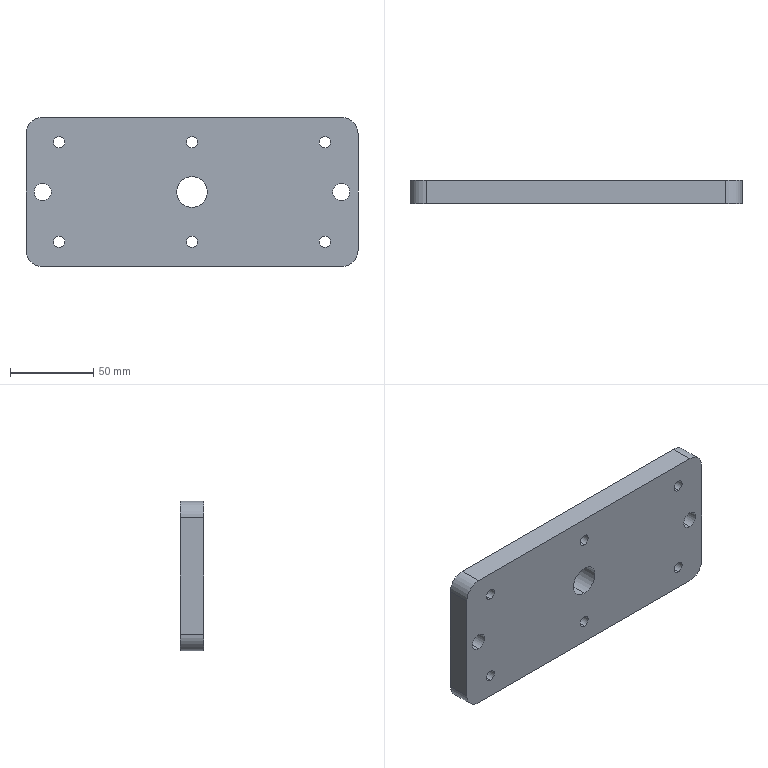Part | SolidWorks | features HoleWzd 4, Extrusion 1, Fillet 1 | 1 solid | 28 faces | box 200 x 14 x 90 mm | volume 241696 mm3 | cylinder 22 | plane 6 | commonest cylinder face diameters 6.8 x12 10.2 x4 20 x4 18.5 x2
STEP:
#1=CARTESIAN_POINT('',(20.,0.,-78.4));
#2=VERTEX_POINT('',#1);
#3=CARTESIAN_POINT('',(20.,0.,-71.6));
#4=VERTEX_POINT('',#3);
#5=CARTESIAN_POINT('',(20.,0.,-75.));
#6=DIRECTION('',(0.,1.,0.));
#7=DIRECTION('',(0.,0.,1.));
#8=AXIS2_PLACEMENT_3D('',#5,#6,#7);
#9=CIRCLE('',#8,3.4);
#10=EDGE_CURVE('',#2,#4,#9,.T.);
#11=ORIENTED_EDGE('',*,*,#10,.F.);
#12=CARTESIAN_POINT('',(20.,14.,-78.4));
#13=VERTEX_POINT('',#12);
#14=CARTESIAN_POINT('',(20.,14.,-78.4));
#15=DIRECTION('',(0.,1.,0.));
#16=VECTOR('',#15,1000.);
#17=LINE('',#14,#16);
#18=EDGE_CURVE('',#2,#13,#17,.T.);
#19=ORIENTED_EDGE('',*,*,#18,.T.);
#20=CARTESIAN_POINT('',(20.,14.,-71.6));
#21=VERTEX_POINT('',#20);
#22=CARTESIAN_POINT('',(20.,14.,-75.));
#23=DIRECTION('',(0.,1.,0.));
#24=DIRECTION('',(0.,0.,1.));
#25=AXIS2_PLACEMENT_3D('',#22,#23,#24);
#26=CIRCLE('',#25,3.4);
#27=EDGE_CURVE('',#13,#21,#26,.T.);
#28=ORIENTED_EDGE('',*,*,#27,.T.);
#29=CARTESIAN_POINT('',(20.,14.,-71.6));
#30=DIRECTION('',(0.,1.,0.));
#31=VECTOR('',#30,1000.);
#32=LINE('',#29,#31);
#33=EDGE_CURVE('',#4,#21,#32,.T.);
#34=ORIENTED_EDGE('',*,*,#33,.F.);
#35=EDGE_LOOP('',(#11,#19,#28,#34));
#36=FACE_OUTER_BOUND('',#35,.T.);
#37=CARTESIAN_POINT('',(20.,14.,-75.));
#38=DIRECTION('',(0.,1.,0.));
#39=DIRECTION('',(0.,0.,1.));
#40=AXIS2_PLACEMENT_3D('',#37,#38,#39);
#41=CYLINDRICAL_SURFACE('',#40,3.4);
#42=ADVANCED_FACE('',(#36),#41,.F.);
#43=CARTESIAN_POINT('',(100.,0.,-78.4));
#44=VERTEX_POINT('',#43);
#45=CARTESIAN_POINT('',(100.,0.,-71.6));
#46=VERTEX_POINT('',#45);
#47=CARTESIAN_POINT('',(100.,0.,-75.));
#48=DIRECTION('',(0.,1.,0.));
#49=DIRECTION('',(0.,0.,1.));
#50=AXIS2_PLACEMENT_3D('',#47,#48,#49);
#51=CIRCLE('',#50,3.4);
#52=EDGE_CURVE('',#44,#46,#51,.T.);
#53=ORIENTED_EDGE('',*,*,#52,.F.);
#54=CARTESIAN_POINT('',(100.,14.,-78.4));
#55=VERTEX_POINT('',#54);
#56=CARTESIAN_POINT('',(100.,14.,-78.4));
#57=DIRECTION('',(0.,1.,0.));
#58=VECTOR('',#57,1000.);
#59=LINE('',#56,#58);
#60=EDGE_CURVE('',#44,#55,#59,.T.);
#61=ORIENTED_EDGE('',*,*,#60,.T.);
#62=CARTESIAN_POINT('',(100.,14.,-71.6));
#63=VERTEX_POINT('',#62);
#64=CARTESIAN_POINT('',(100.,14.,-75.));
#65=DIRECTION('',(0.,1.,0.));
#66=DIRECTION('',(0.,0.,1.));
#67=AXIS2_PLACEMENT_3D('',#64,#65,#66);
#68=CIRCLE('',#67,3.4);
#69=EDGE_CURVE('',#55,#63,#68,.T.);
#70=ORIENTED_EDGE('',*,*,#69,.T.);
#71=CARTESIAN_POINT('',(100.,14.,-71.6));
#72=DIRECTION('',(0.,1.,0.));
#73=VECTOR('',#72,1000.);
#74=LINE('',#71,#73);
#75=EDGE_CURVE('',#46,#63,#74,.T.);
#76=ORIENTED_EDGE('',*,*,#75,.F.);
#77=EDGE_LOOP('',(#53,#61,#70,#76));
#78=FACE_OUTER_BOUND('',#77,.T.);
#79=CARTESIAN_POINT('',(100.,14.,-75.));
#80=DIRECTION('',(0.,1.,0.));
#81=DIRECTION('',(0.,0.,1.));
#82=AXIS2_PLACEMENT_3D('',#79,#80,#81);
#83=CYLINDRICAL_SURFACE('',#82,3.4);
#84=ADVANCED_FACE('',(#78),#83,.F.);
#85=CARTESIAN_POINT('',(180.,0.,-78.4));
#86=VERTEX_POINT('',#85);
#87=CARTESIAN_POINT('',(180.,0.,-71.6));
#88=VERTEX_POINT('',#87);
#89=CARTESIAN_POINT('',(180.,0.,-75.));
#90=DIRECTION('',(0.,1.,0.));
#91=DIRECTION('',(0.,0.,1.));
#92=AXIS2_PLACEMENT_3D('',#89,#90,#91);
#93=CIRCLE('',#92,3.4);
#94=EDGE_CURVE('',#86,#88,#93,.T.);
#95=ORIENTED_EDGE('',*,*,#94,.F.);
#96=CARTESIAN_POINT('',(180.,14.,-78.4));
#97=VERTEX_POINT('',#96);
#98=CARTESIAN_POINT('',(180.,14.,-78.4));
#99=DIRECTION('',(0.,1.,0.));
#100=VECTOR('',#99,1000.);
#101=LINE('',#98,#100);
#102=EDGE_CURVE('',#86,#97,#101,.T.);
#103=ORIENTED_EDGE('',*,*,#102,.T.);
#104=CARTESIAN_POINT('',(180.,14.,-71.6));
#105=VERTEX_POINT('',#104);
#106=CARTESIAN_POINT('',(180.,14.,-75.));
#107=DIRECTION('',(0.,1.,0.));
#108=DIRECTION('',(0.,0.,1.));
#109=AXIS2_PLACEMENT_3D('',#106,#107,#108);
#110=CIRCLE('',#109,3.4);
#111=EDGE_CURVE('',#97,#105,#110,.T.);
#112=ORIENTED_EDGE('',*,*,#111,.T.);
#113=CARTESIAN_POINT('',(180.,14.,-71.6));
#114=DIRECTION('',(0.,1.,0.));
#115=VECTOR('',#114,1000.);
#116=LINE('',#113,#115);
#117=EDGE_CURVE('',#88,#105,#116,.T.);
#118=ORIENTED_EDGE('',*,*,#117,.F.);
#119=EDGE_LOOP('',(#95,#103,#112,#118));
#120=FACE_OUTER_BOUND('',#119,.T.);
#121=CARTESIAN_POINT('',(180.,14.,-75.));
#122=DIRECTION('',(0.,1.,0.));
#123=DIRECTION('',(0.,0.,1.));
#124=AXIS2_PLACEMENT_3D('',#121,#122,#123);
#125=CYLINDRICAL_SURFACE('',#124,3.4);
#126=ADVANCED_FACE('',(#120),#125,.F.);
#127=CARTESIAN_POINT('',(180.,0.,-18.4));
#128=VERTEX_POINT('',#127);
#129=CARTESIAN_POINT('',(180.,0.,-11.6));
#130=VERTEX_POINT('',#129);
#131=CARTESIAN_POINT('',(180.,0.,-15.));
#132=DIRECTION('',(0.,1.,0.));
#133=DIRECTION('',(0.,0.,1.));
#134=AXIS2_PLACEMENT_3D('',#131,#132,#133);
#135=CIRCLE('',#134,3.4);
#136=EDGE_CURVE('',#128,#130,#135,.T.);
#137=ORIENTED_EDGE('',*,*,#136,.F.);
#138=CARTESIAN_POINT('',(180.,14.,-18.4));
#139=VERTEX_POINT('',#138);
#140=CARTESIAN_POINT('',(180.,14.,-18.4));
#141=DIRECTION('',(0.,1.,0.));
#142=VECTOR('',#141,1000.);
#143=LINE('',#140,#142);
#144=EDGE_CURVE('',#128,#139,#143,.T.);
#145=ORIENTED_EDGE('',*,*,#144,.T.);
#146=CARTESIAN_POINT('',(180.,14.,-11.6));
#147=VERTEX_POINT('',#146);
#148=CARTESIAN_POINT('',(180.,14.,-15.));
#149=DIRECTION('',(0.,1.,0.));
#150=DIRECTION('',(0.,0.,1.));
#151=AXIS2_PLACEMENT_3D('',#148,#149,#150);
#152=CIRCLE('',#151,3.4);
#153=EDGE_CURVE('',#139,#147,#152,.T.);
#154=ORIENTED_EDGE('',*,*,#153,.T.);
#155=CARTESIAN_POINT('',(180.,14.,-11.6));
#156=DIRECTION('',(0.,1.,0.));
#157=VECTOR('',#156,1000.);
#158=LINE('',#155,#157);
#159=EDGE_CURVE('',#130,#147,#158,.T.);
#160=ORIENTED_EDGE('',*,*,#159,.F.);
#161=EDGE_LOOP('',(#137,#145,#154,#160));
#162=FACE_OUTER_BOUND('',#161,.T.);
#163=CARTESIAN_POINT('',(180.,14.,-15.));
#164=DIRECTION('',(0.,1.,0.));
#165=DIRECTION('',(0.,0.,1.));
#166=AXIS2_PLACEMENT_3D('',#163,#164,#165);
#167=CYLINDRICAL_SURFACE('',#166,3.4);
#168=ADVANCED_FACE('',(#162),#167,.F.);
#169=CARTESIAN_POINT('',(100.,0.,-18.4));
#170=VERTEX_POINT('',#169);
#171=CARTESIAN_POINT('',(100.,0.,-11.6));
#172=VERTEX_POINT('',#171);
#173=CARTESIAN_POINT('',(100.,0.,-15.));
#174=DIRECTION('',(0.,1.,0.));
#175=DIRECTION('',(0.,0.,1.));
#176=AXIS2_PLACEMENT_3D('',#173,#174,#175);
#177=CIRCLE('',#176,3.4);
#178=EDGE_CURVE('',#170,#172,#177,.T.);
#179=ORIENTED_EDGE('',*,*,#178,.F.);
#180=CARTESIAN_POINT('',(100.,14.,-18.4));
#181=VERTEX_POINT('',#180);
#182=CARTESIAN_POINT('',(100.,14.,-18.4));
#183=DIRECTION('',(0.,1.,0.));
#184=VECTOR('',#183,1000.);
#185=LINE('',#182,#184);
#186=EDGE_CURVE('',#170,#181,#185,.T.);
#187=ORIENTED_EDGE('',*,*,#186,.T.);
#188=CARTESIAN_POINT('',(100.,14.,-11.6));
#189=VERTEX_POINT('',#188);
#190=CARTESIAN_POINT('',(100.,14.,-15.));
#191=DIRECTION('',(0.,1.,0.));
#192=DIRECTION('',(0.,0.,1.));
#193=AXIS2_PLACEMENT_3D('',#190,#191,#192);
#194=CIRCLE('',#193,3.4);
#195=EDGE_CURVE('',#181,#189,#194,.T.);
#196=ORIENTED_EDGE('',*,*,#195,.T.);
#197=CARTESIAN_POINT('',(100.,14.,-11.6));
#198=DIRECTION('',(0.,1.,0.));
#199=VECTOR('',#198,1000.);
#200=LINE('',#197,#199);
#201=EDGE_CURVE('',#172,#189,#200,.T.);
#202=ORIENTED_EDGE('',*,*,#201,.F.);
#203=EDGE_LOOP('',(#179,#187,#196,#202));
#204=FACE_OUTER_BOUND('',#203,.T.);
#205=CARTESIAN_POINT('',(100.,14.,-15.));
#206=DIRECTION('',(0.,1.,0.));
#207=DIRECTION('',(0.,0.,1.));
#208=AXIS2_PLACEMENT_3D('',#205,#206,#207);
#209=CYLINDRICAL_SURFACE('',#208,3.4);
#210=ADVANCED_FACE('',(#204),#209,.F.);
#211=CARTESIAN_POINT('',(20.,0.,-18.4));
#212=VERTEX_POINT('',#211);
#213=CARTESIAN_POINT('',(20.,0.,-11.6));
#214=VERTEX_POINT('',#213);
#215=CARTESIAN_POINT('',(20.,0.,-15.));
#216=DIRECTION('',(0.,1.,0.));
#217=DIRECTION('',(0.,0.,1.));
#218=AXIS2_PLACEMENT_3D('',#215,#216,#217);
#219=CIRCLE('',#218,3.4);
#220=EDGE_CURVE('',#212,#214,#219,.T.);
#221=ORIENTED_EDGE('',*,*,#220,.F.);
#222=CARTESIAN_POINT('',(20.,14.,-18.4));
#223=VERTEX_POINT('',#222);
#224=CARTESIAN_POINT('',(20.,14.,-18.4));
#225=DIRECTION('',(0.,1.,0.));
#226=VECTOR('',#225,1000.);
#227=LINE('',#224,#226);
#228=EDGE_CURVE('',#212,#223,#227,.T.);
#229=ORIENTED_EDGE('',*,*,#228,.T.);
#230=CARTESIAN_POINT('',(20.,14.,-11.6));
#231=VERTEX_POINT('',#230);
#232=CARTESIAN_POINT('',(20.,14.,-15.));
#233=DIRECTION('',(0.,1.,0.));
#234=DIRECTION('',(0.,0.,1.));
#235=AXIS2_PLACEMENT_3D('',#232,#233,#234);
#236=CIRCLE('',#235,3.4);
#237=EDGE_CURVE('',#223,#231,#236,.T.);
#238=ORIENTED_EDGE('',*,*,#237,.T.);
#239=CARTESIAN_POINT('',(20.,14.,-11.6));
#240=DIRECTION('',(0.,1.,0.));
#241=VECTOR('',#240,1000.);
#242=LINE('',#239,#241);
#243=EDGE_CURVE('',#214,#231,#242,.T.);
#244=ORIENTED_EDGE('',*,*,#243,.F.);
#245=EDGE_LOOP('',(#221,#229,#238,#244));
#246=FACE_OUTER_BOUND('',#245,.T.);
#247=CARTESIAN_POINT('',(20.,14.,-15.));
#248=DIRECTION('',(0.,1.,0.));
#249=DIRECTION('',(0.,0.,1.));
#250=AXIS2_PLACEMENT_3D('',#247,#248,#249);
#251=CYLINDRICAL_SURFACE('',#250,3.4);
#252=ADVANCED_FACE('',(#246),#251,.F.);
#253=CARTESIAN_POINT('',(100.,0.,-54.25));
#254=VERTEX_POINT('',#253);
#255=CARTESIAN_POINT('',(100.,0.,-35.75));
#256=VERTEX_POINT('',#255);
#257=CARTESIAN_POINT('',(100.,0.,-45.));
#258=DIRECTION('',(0.,1.,0.));
#259=DIRECTION('',(0.,0.,1.));
#260=AXIS2_PLACEMENT_3D('',#257,#258,#259);
#261=CIRCLE('',#260,9.25);
#262=EDGE_CURVE('',#254,#256,#261,.T.);
#263=ORIENTED_EDGE('',*,*,#262,.F.);
#264=CARTESIAN_POINT('',(100.,14.,-54.25));
#265=VERTEX_POINT('',#264);
#266=CARTESIAN_POINT('',(100.,14.,-54.25));
#267=DIRECTION('',(0.,1.,0.));
#268=VECTOR('',#267,1000.);
#269=LINE('',#266,#268);
#270=EDGE_CURVE('',#254,#265,#269,.T.);
#271=ORIENTED_EDGE('',*,*,#270,.T.);
#272=CARTESIAN_POINT('',(100.,14.,-35.75));
#273=VERTEX_POINT('',#272);
#274=CARTESIAN_POINT('',(100.,14.,-45.));
#275=DIRECTION('',(0.,1.,0.));
#276=DIRECTION('',(0.,0.,1.));
#277=AXIS2_PLACEMENT_3D('',#274,#275,#276);
#278=CIRCLE('',#277,9.25);
#279=EDGE_CURVE('',#265,#273,#278,.T.);
#280=ORIENTED_EDGE('',*,*,#279,.T.);
#281=CARTESIAN_POINT('',(100.,14.,-35.75));
#282=DIRECTION('',(0.,1.,0.));
#283=VECTOR('',#282,1000.);
#284=LINE('',#281,#283);
#285=EDGE_CURVE('',#256,#273,#284,.T.);
#286=ORIENTED_EDGE('',*,*,#285,.F.);
#287=EDGE_LOOP('',(#263,#271,#280,#286));
#288=FACE_OUTER_BOUND('',#287,.T.);
#289=CARTESIAN_POINT('',(100.,14.,-45.));
#290=DIRECTION('',(0.,1.,0.));
#291=DIRECTION('',(0.,0.,1.));
#292=AXIS2_PLACEMENT_3D('',#289,#290,#291);
#293=CYLINDRICAL_SURFACE('',#292,9.25);
#294=ADVANCED_FACE('',(#288),#293,.F.);
#295=CARTESIAN_POINT('',(10.,0.,-39.9));
#296=VERTEX_POINT('',#295);
#297=CARTESIAN_POINT('',(10.,0.,-50.1));
#298=VERTEX_POINT('',#297);
#299=CARTESIAN_POINT('',(10.,0.,-45.));
#300=DIRECTION('',(0.,-1.,0.));
#301=DIRECTION('',(0.,0.,-1.));
#302=AXIS2_PLACEMENT_3D('',#299,#300,#301);
#303=CIRCLE('',#302,5.1);
#304=EDGE_CURVE('',#296,#298,#303,.T.);
#305=ORIENTED_EDGE('',*,*,#304,.T.);
#306=CARTESIAN_POINT('',(10.,14.,-50.1));
#307=VERTEX_POINT('',#306);
#308=CARTESIAN_POINT('',(10.,14.,-50.1));
#309=DIRECTION('',(0.,1.,0.));
#310=VECTOR('',#309,1000.);
#311=LINE('',#308,#310);
#312=EDGE_CURVE('',#298,#307,#311,.T.);
#313=ORIENTED_EDGE('',*,*,#312,.T.);
#314=CARTESIAN_POINT('',(10.,14.,-39.9));
#315=VERTEX_POINT('',#314);
#316=CARTESIAN_POINT('',(10.,14.,-45.));
#317=DIRECTION('',(0.,1.,0.));
#318=DIRECTION('',(0.,0.,1.));
#319=AXIS2_PLACEMENT_3D('',#316,#317,#318);
#320=CIRCLE('',#319,5.1);
#321=EDGE_CURVE('',#307,#315,#320,.T.);
#322=ORIENTED_EDGE('',*,*,#321,.T.);
#323=CARTESIAN_POINT('',(10.,14.,-39.9));
#324=DIRECTION('',(0.,1.,0.));
#325=VECTOR('',#324,1000.);
#326=LINE('',#323,#325);
#327=EDGE_CURVE('',#296,#315,#326,.T.);
#328=ORIENTED_EDGE('',*,*,#327,.F.);
#329=EDGE_LOOP('',(#305,#313,#322,#328));
#330=FACE_OUTER_BOUND('',#329,.T.);
#331=CARTESIAN_POINT('',(10.,14.,-45.));
#332=DIRECTION('',(0.,1.,0.));
#333=DIRECTION('',(0.,0.,1.));
#334=AXIS2_PLACEMENT_3D('',#331,#332,#333);
#335=CYLINDRICAL_SURFACE('',#334,5.1);
#336=ADVANCED_FACE('',(#330),#335,.F.);
#337=CARTESIAN_POINT('',(190.,0.,-39.9));
#338=VERTEX_POINT('',#337);
#339=CARTESIAN_POINT('',(190.,0.,-50.1));
#340=VERTEX_POINT('',#339);
#341=CARTESIAN_POINT('',(190.,0.,-45.));
#342=DIRECTION('',(0.,-1.,0.));
#343=DIRECTION('',(0.,0.,-1.));
#344=AXIS2_PLACEMENT_3D('',#341,#342,#343);
#345=CIRCLE('',#344,5.1);
#346=EDGE_CURVE('',#338,#340,#345,.T.);
#347=ORIENTED_EDGE('',*,*,#346,.T.);
#348=CARTESIAN_POINT('',(190.,14.,-50.1));
#349=VERTEX_POINT('',#348);
#350=CARTESIAN_POINT('',(190.,14.,-50.1));
#351=DIRECTION('',(0.,1.,0.));
#352=VECTOR('',#351,1000.);
#353=LINE('',#350,#352);
#354=EDGE_CURVE('',#340,#349,#353,.T.);
#355=ORIENTED_EDGE('',*,*,#354,.T.);
#356=CARTESIAN_POINT('',(190.,14.,-39.9));
#357=VERTEX_POINT('',#356);
#358=CARTESIAN_POINT('',(190.,14.,-45.));
#359=DIRECTION('',(0.,1.,0.));
#360=DIRECTION('',(0.,0.,1.));
#361=AXIS2_PLACEMENT_3D('',#358,#359,#360);
#362=CIRCLE('',#361,5.1);
#363=EDGE_CURVE('',#349,#357,#362,.T.);
#364=ORIENTED_EDGE('',*,*,#363,.T.);
#365=CARTESIAN_POINT('',(190.,14.,-39.9));
#366=DIRECTION('',(0.,1.,0.));
#367=VECTOR('',#366,1000.);
#368=LINE('',#365,#367);
#369=EDGE_CURVE('',#338,#357,#368,.T.);
#370=ORIENTED_EDGE('',*,*,#369,.F.);
#371=EDGE_LOOP('',(#347,#355,#364,#370));
#372=FACE_OUTER_BOUND('',#371,.T.);
#373=CARTESIAN_POINT('',(190.,14.,-45.));
#374=DIRECTION('',(0.,1.,0.));
#375=DIRECTION('',(0.,0.,1.));
#376=AXIS2_PLACEMENT_3D('',#373,#374,#375);
#377=CYLINDRICAL_SURFACE('',#376,5.1);
#378=ADVANCED_FACE('',(#372),#377,.F.);
#379=CARTESIAN_POINT('',(0.,14.,-80.));
#380=VERTEX_POINT('',#379);
#381=CARTESIAN_POINT('',(0.,14.,-10.));
#382=VERTEX_POINT('',#381);
#383=CARTESIAN_POINT('',(0.,14.,0.));
#384=DIRECTION('',(0.,0.,1.));
#385=VECTOR('',#384,1000.);
#386=LINE('',#383,#385);
#387=EDGE_CURVE('',#380,#382,#386,.T.);
#388=ORIENTED_EDGE('',*,*,#387,.F.);
#389=CARTESIAN_POINT('',(0.,0.,-80.));
#390=VERTEX_POINT('',#389);
#391=CARTESIAN_POINT('',(0.,14.,-80.));
#392=DIRECTION('',(0.,-1.,0.));
#393=VECTOR('',#392,1000.);
#394=LINE('',#391,#393);
#395=EDGE_CURVE('',#380,#390,#394,.T.);
#396=ORIENTED_EDGE('',*,*,#395,.T.);
#397=CARTESIAN_POINT('',(0.,0.,-10.));
#398=VERTEX_POINT('',#397);
#399=CARTESIAN_POINT('',(0.,0.,0.));
#400=DIRECTION('',(0.,0.,1.));
#401=VECTOR('',#400,1000.);
#402=LINE('',#399,#401);
#403=EDGE_CURVE('',#390,#398,#402,.T.);
#404=ORIENTED_EDGE('',*,*,#403,.T.);
#405=CARTESIAN_POINT('',(0.,14.,-10.));
#406=DIRECTION('',(0.,1.,0.));
#407=VECTOR('',#406,1000.);
#408=LINE('',#405,#407);
#409=EDGE_CURVE('',#398,#382,#408,.T.);
#410=ORIENTED_EDGE('',*,*,#409,.T.);
#411=EDGE_LOOP('',(#388,#396,#404,#410));
#412=FACE_OUTER_BOUND('',#411,.T.);
#413=CARTESIAN_POINT('',(0.,14.,0.));
#414=DIRECTION('',(1.,0.,0.));
#415=DIRECTION('',(0.,0.,-1.));
#416=AXIS2_PLACEMENT_3D('',#413,#414,#415);
#417=PLANE('',#416);
#418=ADVANCED_FACE('',(#412),#417,.F.);
#419=CARTESIAN_POINT('',(10.,0.,0.));
#420=VERTEX_POINT('',#419);
#421=CARTESIAN_POINT('',(190.,0.,0.));
#422=VERTEX_POINT('',#421);
#423=CARTESIAN_POINT('',(0.,0.,0.));
#424=DIRECTION('',(1.,0.,0.));
#425=VECTOR('',#424,1000.);
#426=LINE('',#423,#425);
#427=EDGE_CURVE('',#420,#422,#426,.T.);
#428=ORIENTED_EDGE('',*,*,#427,.T.);
#429=CARTESIAN_POINT('',(190.,14.,0.));
#430=VERTEX_POINT('',#429);
#431=CARTESIAN_POINT('',(190.,14.,0.));
#432=DIRECTION('',(0.,1.,0.));
#433=VECTOR('',#432,1000.);
#434=LINE('',#431,#433);
#435=EDGE_CURVE('',#422,#430,#434,.T.);
#436=ORIENTED_EDGE('',*,*,#435,.T.);
#437=CARTESIAN_POINT('',(10.,14.,0.));
#438=VERTEX_POINT('',#437);
#439=CARTESIAN_POINT('',(0.,14.,0.));
#440=DIRECTION('',(1.,0.,0.));
#441=VECTOR('',#440,1000.);
#442=LINE('',#439,#441);
#443=EDGE_CURVE('',#438,#430,#442,.T.);
#444=ORIENTED_EDGE('',*,*,#443,.F.);
#445=CARTESIAN_POINT('',(10.,14.,0.));
#446=DIRECTION('',(0.,-1.,0.));
#447=VECTOR('',#446,1000.);
#448=LINE('',#445,#447);
#449=EDGE_CURVE('',#438,#420,#448,.T.);
#450=ORIENTED_EDGE('',*,*,#449,.T.);
#451=EDGE_LOOP('',(#428,#436,#444,#450));
#452=FACE_OUTER_BOUND('',#451,.T.);
#453=CARTESIAN_POINT('',(0.,14.,0.));
#454=DIRECTION('',(0.,0.,-1.));
#455=DIRECTION('',(-1.,0.,0.));
#456=AXIS2_PLACEMENT_3D('',#453,#454,#455);
#457=PLANE('',#456);
#458=ADVANCED_FACE('',(#452),#457,.F.);
#459=CARTESIAN_POINT('',(200.,0.,-10.));
#460=VERTEX_POINT('',#459);
#461=CARTESIAN_POINT('',(200.,0.,-80.));
#462=VERTEX_POINT('',#461);
#463=CARTESIAN_POINT('',(200.,0.,0.));
#464=DIRECTION('',(0.,0.,-1.));
#465=VECTOR('',#464,1000.);
#466=LINE('',#463,#465);
#467=EDGE_CURVE('',#460,#462,#466,.T.);
#468=ORIENTED_EDGE('',*,*,#467,.T.);
#469=CARTESIAN_POINT('',(200.,14.,-80.));
#470=VERTEX_POINT('',#469);
#471=CARTESIAN_POINT('',(200.,14.,-80.));
#472=DIRECTION('',(0.,1.,0.));
#473=VECTOR('',#472,1000.);
#474=LINE('',#471,#473);
#475=EDGE_CURVE('',#462,#470,#474,.T.);
#476=ORIENTED_EDGE('',*,*,#475,.T.);
#477=CARTESIAN_POINT('',(200.,14.,-10.));
#478=VERTEX_POINT('',#477);
#479=CARTESIAN_POINT('',(200.,14.,0.));
#480=DIRECTION('',(0.,0.,-1.));
#481=VECTOR('',#480,1000.);
#482=LINE('',#479,#481);
#483=EDGE_CURVE('',#478,#470,#482,.T.);
#484=ORIENTED_EDGE('',*,*,#483,.F.);
#485=CARTESIAN_POINT('',(200.,14.,-10.));
#486=DIRECTION('',(0.,-1.,0.));
#487=VECTOR('',#486,1000.);
#488=LINE('',#485,#487);
#489=EDGE_CURVE('',#478,#460,#488,.T.);
#490=ORIENTED_EDGE('',*,*,#489,.T.);
#491=EDGE_LOOP('',(#468,#476,#484,#490));
#492=FACE_OUTER_BOUND('',#491,.T.);
#493=CARTESIAN_POINT('',(200.,14.,0.));
#494=DIRECTION('',(-1.,0.,0.));
#495=DIRECTION('',(0.,0.,1.));
#496=AXIS2_PLACEMENT_3D('',#493,#494,#495);
#497=PLANE('',#496);
#498=ADVANCED_FACE('',(#492),#497,.F.);
#499=CARTESIAN_POINT('',(190.,14.,-90.));
#500=VERTEX_POINT('',#499);
#501=CARTESIAN_POINT('',(10.,14.,-90.));
#502=VERTEX_POINT('',#501);
#503=CARTESIAN_POINT('',(0.,14.,-90.));
#504=DIRECTION('',(-1.,0.,0.));
#505=VECTOR('',#504,1000.);
#506=LINE('',#503,#505);
#507=EDGE_CURVE('',#500,#502,#506,.T.);
#508=ORIENTED_EDGE('',*,*,#507,.F.);
#509=CARTESIAN_POINT('',(190.,0.,-90.));
#510=VERTEX_POINT('',#509);
#511=CARTESIAN_POINT('',(190.,14.,-90.));
#512=DIRECTION('',(0.,-1.,0.));
#513=VECTOR('',#512,1000.);
#514=LINE('',#511,#513);
#515=EDGE_CURVE('',#500,#510,#514,.T.);
#516=ORIENTED_EDGE('',*,*,#515,.T.);
#517=CARTESIAN_POINT('',(10.,0.,-90.));
#518=VERTEX_POINT('',#517);
#519=CARTESIAN_POINT('',(0.,0.,-90.));
#520=DIRECTION('',(-1.,0.,0.));
#521=VECTOR('',#520,1000.);
#522=LINE('',#519,#521);
#523=EDGE_CURVE('',#510,#518,#522,.T.);
#524=ORIENTED_EDGE('',*,*,#523,.T.);
#525=CARTESIAN_POINT('',(10.,14.,-90.));
#526=DIRECTION('',(0.,1.,0.));
#527=VECTOR('',#526,1000.);
#528=LINE('',#525,#527);
#529=EDGE_CURVE('',#518,#502,#528,.T.);
#530=ORIENTED_EDGE('',*,*,#529,.T.);
#531=EDGE_LOOP('',(#508,#516,#524,#530));
#532=FACE_OUTER_BOUND('',#531,.T.);
#533=CARTESIAN_POINT('',(0.,14.,-90.));
#534=DIRECTION('',(0.,0.,1.));
#535=DIRECTION('',(1.,0.,0.));
#536=AXIS2_PLACEMENT_3D('',#533,#534,#535);
#537=PLANE('',#536);
#538=ADVANCED_FACE('',(#532),#537,.F.);
#539=CARTESIAN_POINT('',(20.,14.,-75.));
#540=DIRECTION('',(0.,1.,0.));
#541=DIRECTION('',(0.,0.,1.));
#542=AXIS2_PLACEMENT_3D('',#539,#540,#541);
#543=CIRCLE('',#542,3.4);
#544=EDGE_CURVE('',#21,#13,#543,.T.);
#545=ORIENTED_EDGE('',*,*,#544,.F.);
#546=ORIENTED_EDGE('',*,*,#27,.F.);
#547=EDGE_LOOP('',(#545,#546));
#548=FACE_BOUND('',#547,.T.);
#549=CARTESIAN_POINT('',(100.,14.,-75.));
#550=DIRECTION('',(0.,1.,0.));
#551=DIRECTION('',(0.,0.,1.));
#552=AXIS2_PLACEMENT_3D('',#549,#550,#551);
#553=CIRCLE('',#552,3.4);
#554=EDGE_CURVE('',#63,#55,#553,.T.);
#555=ORIENTED_EDGE('',*,*,#554,.F.);
#556=ORIENTED_EDGE('',*,*,#69,.F.);
#557=EDGE_LOOP('',(#555,#556));
#558=FACE_BOUND('',#557,.T.);
#559=CARTESIAN_POINT('',(180.,14.,-75.));
#560=DIRECTION('',(0.,1.,0.));
#561=DIRECTION('',(0.,0.,1.));
#562=AXIS2_PLACEMENT_3D('',#559,#560,#561);
#563=CIRCLE('',#562,3.4);
#564=EDGE_CURVE('',#105,#97,#563,.T.);
#565=ORIENTED_EDGE('',*,*,#564,.F.);
#566=ORIENTED_EDGE('',*,*,#111,.F.);
#567=EDGE_LOOP('',(#565,#566));
#568=FACE_BOUND('',#567,.T.);
#569=CARTESIAN_POINT('',(180.,14.,-15.));
#570=DIRECTION('',(0.,1.,0.));
#571=DIRECTION('',(0.,0.,1.));
#572=AXIS2_PLACEMENT_3D('',#569,#570,#571);
#573=CIRCLE('',#572,3.4);
#574=EDGE_CURVE('',#147,#139,#573,.T.);
#575=ORIENTED_EDGE('',*,*,#574,.F.);
#576=ORIENTED_EDGE('',*,*,#153,.F.);
#577=EDGE_LOOP('',(#575,#576));
#578=FACE_BOUND('',#577,.T.);
#579=CARTESIAN_POINT('',(100.,14.,-15.));
#580=DIRECTION('',(0.,1.,0.));
#581=DIRECTION('',(0.,0.,1.));
#582=AXIS2_PLACEMENT_3D('',#579,#580,#581);
#583=CIRCLE('',#582,3.4);
#584=EDGE_CURVE('',#189,#181,#583,.T.);
#585=ORIENTED_EDGE('',*,*,#584,.F.);
#586=ORIENTED_EDGE('',*,*,#195,.F.);
#587=EDGE_LOOP('',(#585,#586));
#588=FACE_BOUND('',#587,.T.);
#589=CARTESIAN_POINT('',(20.,14.,-15.));
#590=DIRECTION('',(0.,1.,0.));
#591=DIRECTION('',(0.,0.,1.));
#592=AXIS2_PLACEMENT_3D('',#589,#590,#591);
#593=CIRCLE('',#592,3.4);
#594=EDGE_CURVE('',#231,#223,#593,.T.);
#595=ORIENTED_EDGE('',*,*,#594,.F.);
#596=ORIENTED_EDGE('',*,*,#237,.F.);
#597=EDGE_LOOP('',(#595,#596));
#598=FACE_BOUND('',#597,.T.);
#599=CARTESIAN_POINT('',(100.,14.,-45.));
#600=DIRECTION('',(0.,1.,0.));
#601=DIRECTION('',(0.,0.,1.));
#602=AXIS2_PLACEMENT_3D('',#599,#600,#601);
#603=CIRCLE('',#602,9.25);
#604=EDGE_CURVE('',#273,#265,#603,.T.);
#605=ORIENTED_EDGE('',*,*,#604,.F.);
#606=ORIENTED_EDGE('',*,*,#279,.F.);
#607=EDGE_LOOP('',(#605,#606));
#608=FACE_BOUND('',#607,.T.);
#609=CARTESIAN_POINT('',(10.,14.,-45.));
#610=DIRECTION('',(0.,1.,0.));
#611=DIRECTION('',(0.,0.,1.));
#612=AXIS2_PLACEMENT_3D('',#609,#610,#611);
#613=CIRCLE('',#612,5.1);
#614=EDGE_CURVE('',#315,#307,#613,.T.);
#615=ORIENTED_EDGE('',*,*,#614,.F.);
#616=ORIENTED_EDGE('',*,*,#321,.F.);
#617=EDGE_LOOP('',(#615,#616));
#618=FACE_BOUND('',#617,.T.);
#619=CARTESIAN_POINT('',(190.,14.,-45.));
#620=DIRECTION('',(0.,1.,0.));
#621=DIRECTION('',(0.,0.,1.));
#622=AXIS2_PLACEMENT_3D('',#619,#620,#621);
#623=CIRCLE('',#622,5.1);
#624=EDGE_CURVE('',#357,#349,#623,.T.);
#625=ORIENTED_EDGE('',*,*,#624,.F.);
#626=ORIENTED_EDGE('',*,*,#363,.F.);
#627=EDGE_LOOP('',(#625,#626));
#628=FACE_BOUND('',#627,.T.);
#629=ORIENTED_EDGE('',*,*,#483,.T.);
#630=CARTESIAN_POINT('',(190.,14.,-80.));
#631=DIRECTION('',(0.,1.,0.));
#632=DIRECTION('',(0.,0.,-1.));
#633=AXIS2_PLACEMENT_3D('',#630,#631,#632);
#634=CIRCLE('',#633,10.);
#635=EDGE_CURVE('',#470,#500,#634,.T.);
#636=ORIENTED_EDGE('',*,*,#635,.T.);
#637=ORIENTED_EDGE('',*,*,#507,.T.);
#638=CARTESIAN_POINT('',(10.,14.,-80.));
#639=DIRECTION('',(0.,1.,0.));
#640=DIRECTION('',(0.,0.,-1.));
#641=AXIS2_PLACEMENT_3D('',#638,#639,#640);
#642=CIRCLE('',#641,10.);
#643=EDGE_CURVE('',#502,#380,#642,.T.);
#644=ORIENTED_EDGE('',*,*,#643,.T.);
#645=ORIENTED_EDGE('',*,*,#387,.T.);
#646=CARTESIAN_POINT('',(10.,14.,-10.));
#647=DIRECTION('',(0.,1.,0.));
#648=DIRECTION('',(0.,0.,-1.));
#649=AXIS2_PLACEMENT_3D('',#646,#647,#648);
#650=CIRCLE('',#649,10.);
#651=EDGE_CURVE('',#382,#438,#650,.T.);
#652=ORIENTED_EDGE('',*,*,#651,.T.);
#653=ORIENTED_EDGE('',*,*,#443,.T.);
#654=CARTESIAN_POINT('',(190.,14.,-10.));
#655=DIRECTION('',(0.,1.,0.));
#656=DIRECTION('',(0.,0.,-1.));
#657=AXIS2_PLACEMENT_3D('',#654,#655,#656);
#658=CIRCLE('',#657,10.);
#659=EDGE_CURVE('',#430,#478,#658,.T.);
#660=ORIENTED_EDGE('',*,*,#659,.T.);
#661=EDGE_LOOP('',(#629,#636,#637,#644,#645,#652,#653,#660));
#662=FACE_OUTER_BOUND('',#661,.T.);
#663=CARTESIAN_POINT('',(0.,14.,0.));
#664=DIRECTION('',(0.,-1.,0.));
#665=DIRECTION('',(0.,0.,-1.));
#666=AXIS2_PLACEMENT_3D('',#663,#664,#665);
#667=PLANE('',#666);
#668=ADVANCED_FACE('',(#548,#558,#568,#578,#588,#598,#608,#618,#628,#662),#667,.F.);
#669=CARTESIAN_POINT('',(20.,0.,-75.));
#670=DIRECTION('',(0.,1.,0.));
#671=DIRECTION('',(0.,0.,1.));
#672=AXIS2_PLACEMENT_3D('',#669,#670,#671);
#673=CIRCLE('',#672,3.4);
#674=EDGE_CURVE('',#4,#2,#673,.T.);
#675=ORIENTED_EDGE('',*,*,#674,.T.);
#676=ORIENTED_EDGE('',*,*,#10,.T.);
#677=EDGE_LOOP('',(#675,#676));
#678=FACE_BOUND('',#677,.T.);
#679=CARTESIAN_POINT('',(100.,0.,-75.));
#680=DIRECTION('',(0.,1.,0.));
#681=DIRECTION('',(0.,0.,1.));
#682=AXIS2_PLACEMENT_3D('',#679,#680,#681);
#683=CIRCLE('',#682,3.4);
#684=EDGE_CURVE('',#46,#44,#683,.T.);
#685=ORIENTED_EDGE('',*,*,#684,.T.);
#686=ORIENTED_EDGE('',*,*,#52,.T.);
#687=EDGE_LOOP('',(#685,#686));
#688=FACE_BOUND('',#687,.T.);
#689=CARTESIAN_POINT('',(180.,0.,-75.));
#690=DIRECTION('',(0.,1.,0.));
#691=DIRECTION('',(0.,0.,1.));
#692=AXIS2_PLACEMENT_3D('',#689,#690,#691);
#693=CIRCLE('',#692,3.4);
#694=EDGE_CURVE('',#88,#86,#693,.T.);
#695=ORIENTED_EDGE('',*,*,#694,.T.);
#696=ORIENTED_EDGE('',*,*,#94,.T.);
#697=EDGE_LOOP('',(#695,#696));
#698=FACE_BOUND('',#697,.T.);
#699=CARTESIAN_POINT('',(180.,0.,-15.));
#700=DIRECTION('',(0.,1.,0.));
#701=DIRECTION('',(0.,0.,1.));
#702=AXIS2_PLACEMENT_3D('',#699,#700,#701);
#703=CIRCLE('',#702,3.4);
#704=EDGE_CURVE('',#130,#128,#703,.T.);
#705=ORIENTED_EDGE('',*,*,#704,.T.);
#706=ORIENTED_EDGE('',*,*,#136,.T.);
#707=EDGE_LOOP('',(#705,#706));
#708=FACE_BOUND('',#707,.T.);
#709=CARTESIAN_POINT('',(100.,0.,-15.));
#710=DIRECTION('',(0.,1.,0.));
#711=DIRECTION('',(0.,0.,1.));
#712=AXIS2_PLACEMENT_3D('',#709,#710,#711);
#713=CIRCLE('',#712,3.4);
#714=EDGE_CURVE('',#172,#170,#713,.T.);
#715=ORIENTED_EDGE('',*,*,#714,.T.);
#716=ORIENTED_EDGE('',*,*,#178,.T.);
#717=EDGE_LOOP('',(#715,#716));
#718=FACE_BOUND('',#717,.T.);
#719=CARTESIAN_POINT('',(20.,0.,-15.));
#720=DIRECTION('',(0.,1.,0.));
#721=DIRECTION('',(0.,0.,1.));
#722=AXIS2_PLACEMENT_3D('',#719,#720,#721);
#723=CIRCLE('',#722,3.4);
#724=EDGE_CURVE('',#214,#212,#723,.T.);
#725=ORIENTED_EDGE('',*,*,#724,.T.);
#726=ORIENTED_EDGE('',*,*,#220,.T.);
#727=EDGE_LOOP('',(#725,#726));
#728=FACE_BOUND('',#727,.T.);
#729=CARTESIAN_POINT('',(100.,0.,-45.));
#730=DIRECTION('',(0.,1.,0.));
#731=DIRECTION('',(0.,0.,1.));
#732=AXIS2_PLACEMENT_3D('',#729,#730,#731);
#733=CIRCLE('',#732,9.25);
#734=EDGE_CURVE('',#256,#254,#733,.T.);
#735=ORIENTED_EDGE('',*,*,#734,.T.);
#736=ORIENTED_EDGE('',*,*,#262,.T.);
#737=EDGE_LOOP('',(#735,#736));
#738=FACE_BOUND('',#737,.T.);
#739=ORIENTED_EDGE('',*,*,#304,.F.);
#740=CARTESIAN_POINT('',(10.,0.,-45.));
#741=DIRECTION('',(0.,-1.,0.));
#742=DIRECTION('',(0.,0.,-1.));
#743=AXIS2_PLACEMENT_3D('',#740,#741,#742);
#744=CIRCLE('',#743,5.1);
#745=EDGE_CURVE('',#298,#296,#744,.T.);
#746=ORIENTED_EDGE('',*,*,#745,.F.);
#747=EDGE_LOOP('',(#739,#746));
#748=FACE_BOUND('',#747,.T.);
#749=ORIENTED_EDGE('',*,*,#346,.F.);
#750=CARTESIAN_POINT('',(190.,0.,-45.));
#751=DIRECTION('',(0.,-1.,0.));
#752=DIRECTION('',(0.,0.,-1.));
#753=AXIS2_PLACEMENT_3D('',#750,#751,#752);
#754=CIRCLE('',#753,5.1);
#755=EDGE_CURVE('',#340,#338,#754,.T.);
#756=ORIENTED_EDGE('',*,*,#755,.F.);
#757=EDGE_LOOP('',(#749,#756));
#758=FACE_BOUND('',#757,.T.);
#759=ORIENTED_EDGE('',*,*,#523,.F.);
#760=CARTESIAN_POINT('',(190.,0.,-80.));
#761=DIRECTION('',(0.,-1.,0.));
#762=DIRECTION('',(0.,0.,-1.));
#763=AXIS2_PLACEMENT_3D('',#760,#761,#762);
#764=CIRCLE('',#763,10.);
#765=EDGE_CURVE('',#510,#462,#764,.T.);
#766=ORIENTED_EDGE('',*,*,#765,.T.);
#767=ORIENTED_EDGE('',*,*,#467,.F.);
#768=CARTESIAN_POINT('',(190.,0.,-10.));
#769=DIRECTION('',(0.,-1.,0.));
#770=DIRECTION('',(0.,0.,-1.));
#771=AXIS2_PLACEMENT_3D('',#768,#769,#770);
#772=CIRCLE('',#771,10.);
#773=EDGE_CURVE('',#460,#422,#772,.T.);
#774=ORIENTED_EDGE('',*,*,#773,.T.);
#775=ORIENTED_EDGE('',*,*,#427,.F.);
#776=CARTESIAN_POINT('',(10.,0.,-10.));
#777=DIRECTION('',(0.,-1.,0.));
#778=DIRECTION('',(0.,0.,-1.));
#779=AXIS2_PLACEMENT_3D('',#776,#777,#778);
#780=CIRCLE('',#779,10.);
#781=EDGE_CURVE('',#420,#398,#780,.T.);
#782=ORIENTED_EDGE('',*,*,#781,.T.);
#783=ORIENTED_EDGE('',*,*,#403,.F.);
#784=CARTESIAN_POINT('',(10.,0.,-80.));
#785=DIRECTION('',(0.,-1.,0.));
#786=DIRECTION('',(0.,0.,-1.));
#787=AXIS2_PLACEMENT_3D('',#784,#785,#786);
#788=CIRCLE('',#787,10.);
#789=EDGE_CURVE('',#390,#518,#788,.T.);
#790=ORIENTED_EDGE('',*,*,#789,.T.);
#791=EDGE_LOOP('',(#759,#766,#767,#774,#775,#782,#783,#790));
#792=FACE_OUTER_BOUND('',#791,.T.);
#793=CARTESIAN_POINT('',(0.,0.,0.));
#794=DIRECTION('',(0.,-1.,0.));
#795=DIRECTION('',(0.,0.,-1.));
#796=AXIS2_PLACEMENT_3D('',#793,#794,#795);
#797=PLANE('',#796);
#798=ADVANCED_FACE('',(#678,#688,#698,#708,#718,#728,#738,#748,#758,#792),#797,.T.);
#799=ORIENTED_EDGE('',*,*,#354,.F.);
#800=ORIENTED_EDGE('',*,*,#755,.T.);
#801=ORIENTED_EDGE('',*,*,#369,.T.);
#802=ORIENTED_EDGE('',*,*,#624,.T.);
#803=EDGE_LOOP('',(#799,#800,#801,#802));
#804=FACE_OUTER_BOUND('',#803,.T.);
#805=CARTESIAN_POINT('',(190.,14.,-45.));
#806=DIRECTION('',(0.,1.,0.));
#807=DIRECTION('',(0.,0.,1.));
#808=AXIS2_PLACEMENT_3D('',#805,#806,#807);
#809=CYLINDRICAL_SURFACE('',#808,5.1);
#810=ADVANCED_FACE('',(#804),#809,.F.);
#811=ORIENTED_EDGE('',*,*,#312,.F.);
#812=ORIENTED_EDGE('',*,*,#745,.T.);
#813=ORIENTED_EDGE('',*,*,#327,.T.);
#814=ORIENTED_EDGE('',*,*,#614,.T.);
#815=EDGE_LOOP('',(#811,#812,#813,#814));
#816=FACE_OUTER_BOUND('',#815,.T.);
#817=CARTESIAN_POINT('',(10.,14.,-45.));
#818=DIRECTION('',(0.,1.,0.));
#819=DIRECTION('',(0.,0.,1.));
#820=AXIS2_PLACEMENT_3D('',#817,#818,#819);
#821=CYLINDRICAL_SURFACE('',#820,5.1);
#822=ADVANCED_FACE('',(#816),#821,.F.);
#823=ORIENTED_EDGE('',*,*,#635,.F.);
#824=ORIENTED_EDGE('',*,*,#475,.F.);
#825=ORIENTED_EDGE('',*,*,#765,.F.);
#826=ORIENTED_EDGE('',*,*,#515,.F.);
#827=EDGE_LOOP('',(#823,#824,#825,#826));
#828=FACE_OUTER_BOUND('',#827,.T.);
#829=CARTESIAN_POINT('',(190.,14.,-80.));
#830=DIRECTION('',(0.,-1.,0.));
#831=DIRECTION('',(0.,0.,-1.));
#832=AXIS2_PLACEMENT_3D('',#829,#830,#831);
#833=CYLINDRICAL_SURFACE('',#832,10.);
#834=ADVANCED_FACE('',(#828),#833,.T.);
#835=ORIENTED_EDGE('',*,*,#659,.F.);
#836=ORIENTED_EDGE('',*,*,#435,.F.);
#837=ORIENTED_EDGE('',*,*,#773,.F.);
#838=ORIENTED_EDGE('',*,*,#489,.F.);
#839=EDGE_LOOP('',(#835,#836,#837,#838));
#840=FACE_OUTER_BOUND('',#839,.T.);
#841=CARTESIAN_POINT('',(190.,14.,-10.));
#842=DIRECTION('',(0.,-1.,0.));
#843=DIRECTION('',(0.,0.,-1.));
#844=AXIS2_PLACEMENT_3D('',#841,#842,#843);
#845=CYLINDRICAL_SURFACE('',#844,10.);
#846=ADVANCED_FACE('',(#840),#845,.T.);
#847=ORIENTED_EDGE('',*,*,#643,.F.);
#848=ORIENTED_EDGE('',*,*,#529,.F.);
#849=ORIENTED_EDGE('',*,*,#789,.F.);
#850=ORIENTED_EDGE('',*,*,#395,.F.);
#851=EDGE_LOOP('',(#847,#848,#849,#850));
#852=FACE_OUTER_BOUND('',#851,.T.);
#853=CARTESIAN_POINT('',(10.,14.,-80.));
#854=DIRECTION('',(0.,-1.,0.));
#855=DIRECTION('',(0.,0.,-1.));
#856=AXIS2_PLACEMENT_3D('',#853,#854,#855);
#857=CYLINDRICAL_SURFACE('',#856,10.);
#858=ADVANCED_FACE('',(#852),#857,.T.);
#859=ORIENTED_EDGE('',*,*,#651,.F.);
#860=ORIENTED_EDGE('',*,*,#409,.F.);
#861=ORIENTED_EDGE('',*,*,#781,.F.);
#862=ORIENTED_EDGE('',*,*,#449,.F.);
#863=EDGE_LOOP('',(#859,#860,#861,#862));
#864=FACE_OUTER_BOUND('',#863,.T.);
#865=CARTESIAN_POINT('',(10.,14.,-10.));
#866=DIRECTION('',(0.,-1.,0.));
#867=DIRECTION('',(0.,0.,-1.));
#868=AXIS2_PLACEMENT_3D('',#865,#866,#867);
#869=CYLINDRICAL_SURFACE('',#868,10.);
#870=ADVANCED_FACE('',(#864),#869,.T.);
#871=ORIENTED_EDGE('',*,*,#270,.F.);
#872=ORIENTED_EDGE('',*,*,#734,.F.);
#873=ORIENTED_EDGE('',*,*,#285,.T.);
#874=ORIENTED_EDGE('',*,*,#604,.T.);
#875=EDGE_LOOP('',(#871,#872,#873,#874));
#876=FACE_OUTER_BOUND('',#875,.T.);
#877=CARTESIAN_POINT('',(100.,14.,-45.));
#878=DIRECTION('',(0.,1.,0.));
#879=DIRECTION('',(0.,0.,1.));
#880=AXIS2_PLACEMENT_3D('',#877,#878,#879);
#881=CYLINDRICAL_SURFACE('',#880,9.25);
#882=ADVANCED_FACE('',(#876),#881,.F.);
#883=ORIENTED_EDGE('',*,*,#228,.F.);
#884=ORIENTED_EDGE('',*,*,#724,.F.);
#885=ORIENTED_EDGE('',*,*,#243,.T.);
#886=ORIENTED_EDGE('',*,*,#594,.T.);
#887=EDGE_LOOP('',(#883,#884,#885,#886));
#888=FACE_OUTER_BOUND('',#887,.T.);
#889=CARTESIAN_POINT('',(20.,14.,-15.));
#890=DIRECTION('',(0.,1.,0.));
#891=DIRECTION('',(0.,0.,1.));
#892=AXIS2_PLACEMENT_3D('',#889,#890,#891);
#893=CYLINDRICAL_SURFACE('',#892,3.4);
#894=ADVANCED_FACE('',(#888),#893,.F.);
#895=ORIENTED_EDGE('',*,*,#186,.F.);
#896=ORIENTED_EDGE('',*,*,#714,.F.);
#897=ORIENTED_EDGE('',*,*,#201,.T.);
#898=ORIENTED_EDGE('',*,*,#584,.T.);
#899=EDGE_LOOP('',(#895,#896,#897,#898));
#900=FACE_OUTER_BOUND('',#899,.T.);
#901=CARTESIAN_POINT('',(100.,14.,-15.));
#902=DIRECTION('',(0.,1.,0.));
#903=DIRECTION('',(0.,0.,1.));
#904=AXIS2_PLACEMENT_3D('',#901,#902,#903);
#905=CYLINDRICAL_SURFACE('',#904,3.4);
#906=ADVANCED_FACE('',(#900),#905,.F.);
#907=ORIENTED_EDGE('',*,*,#144,.F.);
#908=ORIENTED_EDGE('',*,*,#704,.F.);
#909=ORIENTED_EDGE('',*,*,#159,.T.);
#910=ORIENTED_EDGE('',*,*,#574,.T.);
#911=EDGE_LOOP('',(#907,#908,#909,#910));
#912=FACE_OUTER_BOUND('',#911,.T.);
#913=CARTESIAN_POINT('',(180.,14.,-15.));
#914=DIRECTION('',(0.,1.,0.));
#915=DIRECTION('',(0.,0.,1.));
#916=AXIS2_PLACEMENT_3D('',#913,#914,#915);
#917=CYLINDRICAL_SURFACE('',#916,3.4);
#918=ADVANCED_FACE('',(#912),#917,.F.);
#919=ORIENTED_EDGE('',*,*,#102,.F.);
#920=ORIENTED_EDGE('',*,*,#694,.F.);
#921=ORIENTED_EDGE('',*,*,#117,.T.);
#922=ORIENTED_EDGE('',*,*,#564,.T.);
#923=EDGE_LOOP('',(#919,#920,#921,#922));
#924=FACE_OUTER_BOUND('',#923,.T.);
#925=CARTESIAN_POINT('',(180.,14.,-75.));
#926=DIRECTION('',(0.,1.,0.));
#927=DIRECTION('',(0.,0.,1.));
#928=AXIS2_PLACEMENT_3D('',#925,#926,#927);
#929=CYLINDRICAL_SURFACE('',#928,3.4);
#930=ADVANCED_FACE('',(#924),#929,.F.);
#931=ORIENTED_EDGE('',*,*,#60,.F.);
#932=ORIENTED_EDGE('',*,*,#684,.F.);
#933=ORIENTED_EDGE('',*,*,#75,.T.);
#934=ORIENTED_EDGE('',*,*,#554,.T.);
#935=EDGE_LOOP('',(#931,#932,#933,#934));
#936=FACE_OUTER_BOUND('',#935,.T.);
#937=CARTESIAN_POINT('',(100.,14.,-75.));
#938=DIRECTION('',(0.,1.,0.));
#939=DIRECTION('',(0.,0.,1.));
#940=AXIS2_PLACEMENT_3D('',#937,#938,#939);
#941=CYLINDRICAL_SURFACE('',#940,3.4);
#942=ADVANCED_FACE('',(#936),#941,.F.);
#943=ORIENTED_EDGE('',*,*,#18,.F.);
#944=ORIENTED_EDGE('',*,*,#674,.F.);
#945=ORIENTED_EDGE('',*,*,#33,.T.);
#946=ORIENTED_EDGE('',*,*,#544,.T.);
#947=EDGE_LOOP('',(#943,#944,#945,#946));
#948=FACE_OUTER_BOUND('',#947,.T.);
#949=CARTESIAN_POINT('',(20.,14.,-75.));
#950=DIRECTION('',(0.,1.,0.));
#951=DIRECTION('',(0.,0.,1.));
#952=AXIS2_PLACEMENT_3D('',#949,#950,#951);
#953=CYLINDRICAL_SURFACE('',#952,3.4);
#954=ADVANCED_FACE('',(#948),#953,.F.);
#955=CLOSED_SHELL('',(#42,#84,#126,#168,#210,#252,#294,#336,#378,#418,#458,#498,#538,#668,#798,#810,#822,#834,#846,#858,#870,#882,#894,#906,#918,#930,#942,#954));
#956=MANIFOLD_SOLID_BREP('',#955);
#957=CARTESIAN_POINT('',(0.,0.,0.));
#958=DIRECTION('',(0.,0.,1.));
#959=DIRECTION('',(1.,0.,0.));
#960=AXIS2_PLACEMENT_3D('',#957,#958,#959);
#961=(LENGTH_UNIT()NAMED_UNIT(*)SI_UNIT(.MILLI.,.METRE.));
#962=UNCERTAINTY_MEASURE_WITH_UNIT(LENGTH_MEASURE(0.00001),#961,'','');
#963=(NAMED_UNIT(*)PLANE_ANGLE_UNIT()SI_UNIT($,.RADIAN.));
#964=(NAMED_UNIT(*)SI_UNIT($,.STERADIAN.)SOLID_ANGLE_UNIT());
#965=(GEOMETRIC_REPRESENTATION_CONTEXT(3)GLOBAL_UNCERTAINTY_ASSIGNED_CONTEXT((#962))GLOBAL_UNIT_ASSIGNED_CONTEXT((#961,#963,#964))REPRESENTATION_CONTEXT('',''));
#966=ADVANCED_BREP_SHAPE_REPRESENTATION('',(#956,#960),#965);